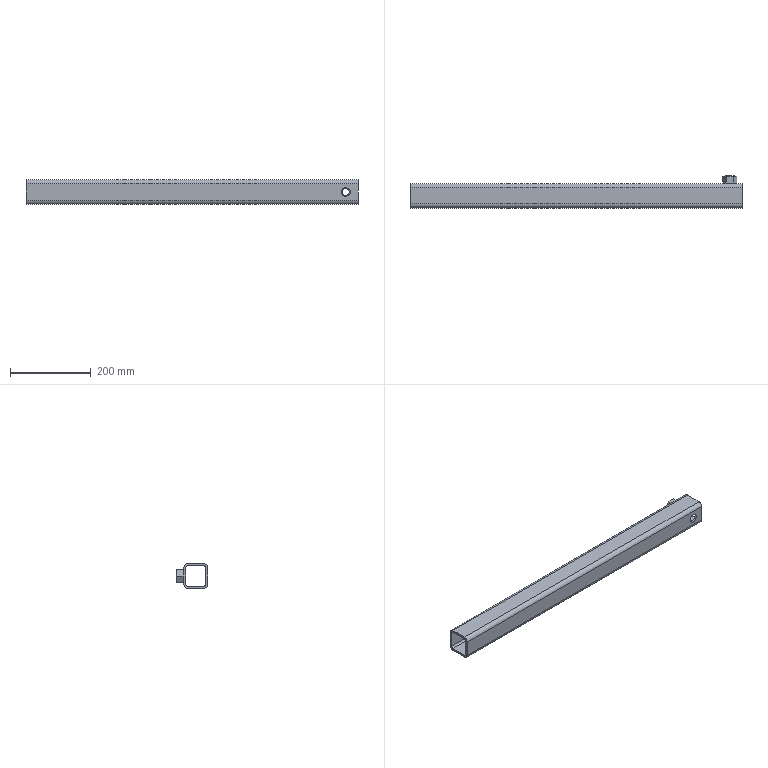Part | 2 solids | 36 faces | box 820 x 79 x 60 mm | volume 855655 mm3 | plane 18 | cylinder 14 | cone 4 | commonest cylinder face diameters 10 x4 20 x4 22 x4 17.294 x2
STEP:
#1=CARTESIAN_POINT('',(790.,25.,11.));
#2=VERTEX_POINT('',#1);
#3=CARTESIAN_POINT('',(790.,25.,-11.));
#4=VERTEX_POINT('',#3);
#5=CARTESIAN_POINT('',(790.,25.,0.));
#6=DIRECTION('',(0.,-1.,0.));
#7=DIRECTION('',(0.,0.,-1.));
#8=AXIS2_PLACEMENT_3D('',#5,#6,#7);
#9=CIRCLE('',#8,11.);
#10=EDGE_CURVE('',#2,#4,#9,.T.);
#11=ORIENTED_EDGE('',*,*,#10,.T.);
#12=CARTESIAN_POINT('',(790.,30.,-11.));
#13=VERTEX_POINT('',#12);
#14=CARTESIAN_POINT('',(790.,30.,-11.));
#15=DIRECTION('',(0.,1.,0.));
#16=VECTOR('',#15,1000.);
#17=LINE('',#14,#16);
#18=EDGE_CURVE('',#4,#13,#17,.T.);
#19=ORIENTED_EDGE('',*,*,#18,.T.);
#20=CARTESIAN_POINT('',(790.,30.,11.));
#21=VERTEX_POINT('',#20);
#22=CARTESIAN_POINT('',(790.,30.,0.));
#23=DIRECTION('',(0.,1.,0.));
#24=DIRECTION('',(0.,0.,1.));
#25=AXIS2_PLACEMENT_3D('',#22,#23,#24);
#26=CIRCLE('',#25,11.);
#27=EDGE_CURVE('',#13,#21,#26,.T.);
#28=ORIENTED_EDGE('',*,*,#27,.T.);
#29=CARTESIAN_POINT('',(790.,30.,11.));
#30=DIRECTION('',(0.,1.,0.));
#31=VECTOR('',#30,1000.);
#32=LINE('',#29,#31);
#33=EDGE_CURVE('',#2,#21,#32,.T.);
#34=ORIENTED_EDGE('',*,*,#33,.F.);
#35=EDGE_LOOP('',(#11,#19,#28,#34));
#36=FACE_OUTER_BOUND('',#35,.T.);
#37=CARTESIAN_POINT('',(790.,30.,0.));
#38=DIRECTION('',(0.,1.,0.));
#39=DIRECTION('',(0.,0.,1.));
#40=AXIS2_PLACEMENT_3D('',#37,#38,#39);
#41=CYLINDRICAL_SURFACE('',#40,11.);
#42=ADVANCED_FACE('',(#36),#41,.F.);
#43=CARTESIAN_POINT('',(790.,-30.,-11.));
#44=VERTEX_POINT('',#43);
#45=CARTESIAN_POINT('',(790.,-30.,11.));
#46=VERTEX_POINT('',#45);
#47=CARTESIAN_POINT('',(790.,-30.,0.));
#48=DIRECTION('',(0.,1.,0.));
#49=DIRECTION('',(0.,0.,1.));
#50=AXIS2_PLACEMENT_3D('',#47,#48,#49);
#51=CIRCLE('',#50,11.);
#52=EDGE_CURVE('',#44,#46,#51,.T.);
#53=ORIENTED_EDGE('',*,*,#52,.F.);
#54=CARTESIAN_POINT('',(790.,-25.,-11.));
#55=VERTEX_POINT('',#54);
#56=CARTESIAN_POINT('',(790.,30.,-11.));
#57=DIRECTION('',(0.,1.,0.));
#58=VECTOR('',#57,1000.);
#59=LINE('',#56,#58);
#60=EDGE_CURVE('',#44,#55,#59,.T.);
#61=ORIENTED_EDGE('',*,*,#60,.T.);
#62=CARTESIAN_POINT('',(790.,-25.,11.));
#63=VERTEX_POINT('',#62);
#64=CARTESIAN_POINT('',(790.,-25.,0.));
#65=DIRECTION('',(0.,1.,0.));
#66=DIRECTION('',(0.,0.,1.));
#67=AXIS2_PLACEMENT_3D('',#64,#65,#66);
#68=CIRCLE('',#67,11.);
#69=EDGE_CURVE('',#55,#63,#68,.T.);
#70=ORIENTED_EDGE('',*,*,#69,.T.);
#71=CARTESIAN_POINT('',(790.,30.,11.));
#72=DIRECTION('',(0.,1.,0.));
#73=VECTOR('',#72,1000.);
#74=LINE('',#71,#73);
#75=EDGE_CURVE('',#46,#63,#74,.T.);
#76=ORIENTED_EDGE('',*,*,#75,.F.);
#77=EDGE_LOOP('',(#53,#61,#70,#76));
#78=FACE_OUTER_BOUND('',#77,.T.);
#79=CARTESIAN_POINT('',(790.,30.,0.));
#80=DIRECTION('',(0.,1.,0.));
#81=DIRECTION('',(0.,0.,1.));
#82=AXIS2_PLACEMENT_3D('',#79,#80,#81);
#83=CYLINDRICAL_SURFACE('',#82,11.);
#84=ADVANCED_FACE('',(#78),#83,.F.);
#85=CARTESIAN_POINT('',(0.,20.,-30.));
#86=VERTEX_POINT('',#85);
#87=CARTESIAN_POINT('',(0.,30.,-20.));
#88=VERTEX_POINT('',#87);
#89=CARTESIAN_POINT('',(0.,20.,-20.));
#90=DIRECTION('',(1.,0.,0.));
#91=DIRECTION('',(0.,0.,-1.));
#92=AXIS2_PLACEMENT_3D('',#89,#90,#91);
#93=CIRCLE('',#92,10.);
#94=EDGE_CURVE('',#86,#88,#93,.T.);
#95=ORIENTED_EDGE('',*,*,#94,.T.);
#96=CARTESIAN_POINT('',(820.,30.,-20.));
#97=VERTEX_POINT('',#96);
#98=CARTESIAN_POINT('',(820.,30.,-20.));
#99=DIRECTION('',(-1.,0.,0.));
#100=VECTOR('',#99,1000.);
#101=LINE('',#98,#100);
#102=EDGE_CURVE('',#97,#88,#101,.T.);
#103=ORIENTED_EDGE('',*,*,#102,.F.);
#104=CARTESIAN_POINT('',(820.,20.,-30.));
#105=VERTEX_POINT('',#104);
#106=CARTESIAN_POINT('',(820.,20.,-20.));
#107=DIRECTION('',(1.,0.,0.));
#108=DIRECTION('',(0.,0.,-1.));
#109=AXIS2_PLACEMENT_3D('',#106,#107,#108);
#110=CIRCLE('',#109,10.);
#111=EDGE_CURVE('',#105,#97,#110,.T.);
#112=ORIENTED_EDGE('',*,*,#111,.F.);
#113=CARTESIAN_POINT('',(820.,20.,-30.));
#114=DIRECTION('',(-1.,0.,0.));
#115=VECTOR('',#114,1000.);
#116=LINE('',#113,#115);
#117=EDGE_CURVE('',#105,#86,#116,.T.);
#118=ORIENTED_EDGE('',*,*,#117,.T.);
#119=EDGE_LOOP('',(#95,#103,#112,#118));
#120=FACE_OUTER_BOUND('',#119,.T.);
#121=CARTESIAN_POINT('',(820.,20.,-20.));
#122=DIRECTION('',(-1.,0.,0.));
#123=DIRECTION('',(0.,0.,1.));
#124=AXIS2_PLACEMENT_3D('',#121,#122,#123);
#125=CYLINDRICAL_SURFACE('',#124,10.);
#126=ADVANCED_FACE('',(#120),#125,.T.);
#127=CARTESIAN_POINT('',(790.,30.,0.));
#128=DIRECTION('',(0.,1.,0.));
#129=DIRECTION('',(0.,0.,1.));
#130=AXIS2_PLACEMENT_3D('',#127,#128,#129);
#131=CIRCLE('',#130,11.);
#132=EDGE_CURVE('',#21,#13,#131,.T.);
#133=ORIENTED_EDGE('',*,*,#132,.F.);
#134=ORIENTED_EDGE('',*,*,#27,.F.);
#135=EDGE_LOOP('',(#133,#134));
#136=FACE_BOUND('',#135,.T.);
#137=CARTESIAN_POINT('',(0.,30.,20.));
#138=VERTEX_POINT('',#137);
#139=CARTESIAN_POINT('',(0.,30.,-20.));
#140=DIRECTION('',(0.,0.,1.));
#141=VECTOR('',#140,1000.);
#142=LINE('',#139,#141);
#143=EDGE_CURVE('',#88,#138,#142,.T.);
#144=ORIENTED_EDGE('',*,*,#143,.T.);
#145=CARTESIAN_POINT('',(820.,30.,20.));
#146=VERTEX_POINT('',#145);
#147=CARTESIAN_POINT('',(820.,30.,20.));
#148=DIRECTION('',(-1.,0.,0.));
#149=VECTOR('',#148,1000.);
#150=LINE('',#147,#149);
#151=EDGE_CURVE('',#146,#138,#150,.T.);
#152=ORIENTED_EDGE('',*,*,#151,.F.);
#153=CARTESIAN_POINT('',(820.,30.,-20.));
#154=DIRECTION('',(0.,0.,1.));
#155=VECTOR('',#154,1000.);
#156=LINE('',#153,#155);
#157=EDGE_CURVE('',#97,#146,#156,.T.);
#158=ORIENTED_EDGE('',*,*,#157,.F.);
#159=ORIENTED_EDGE('',*,*,#102,.T.);
#160=EDGE_LOOP('',(#144,#152,#158,#159));
#161=FACE_OUTER_BOUND('',#160,.T.);
#162=CARTESIAN_POINT('',(820.,30.,-20.));
#163=DIRECTION('',(0.,-1.,0.));
#164=DIRECTION('',(0.,0.,-1.));
#165=AXIS2_PLACEMENT_3D('',#162,#163,#164);
#166=PLANE('',#165);
#167=ADVANCED_FACE('',(#136,#161),#166,.F.);
#168=CARTESIAN_POINT('',(0.,20.,30.));
#169=VERTEX_POINT('',#168);
#170=CARTESIAN_POINT('',(0.,20.,20.));
#171=DIRECTION('',(1.,0.,0.));
#172=DIRECTION('',(0.,0.,-1.));
#173=AXIS2_PLACEMENT_3D('',#170,#171,#172);
#174=CIRCLE('',#173,10.);
#175=EDGE_CURVE('',#138,#169,#174,.T.);
#176=ORIENTED_EDGE('',*,*,#175,.T.);
#177=CARTESIAN_POINT('',(820.,20.,30.));
#178=VERTEX_POINT('',#177);
#179=CARTESIAN_POINT('',(820.,20.,30.));
#180=DIRECTION('',(-1.,0.,0.));
#181=VECTOR('',#180,1000.);
#182=LINE('',#179,#181);
#183=EDGE_CURVE('',#178,#169,#182,.T.);
#184=ORIENTED_EDGE('',*,*,#183,.F.);
#185=CARTESIAN_POINT('',(820.,20.,20.));
#186=DIRECTION('',(1.,0.,0.));
#187=DIRECTION('',(0.,0.,-1.));
#188=AXIS2_PLACEMENT_3D('',#185,#186,#187);
#189=CIRCLE('',#188,10.);
#190=EDGE_CURVE('',#146,#178,#189,.T.);
#191=ORIENTED_EDGE('',*,*,#190,.F.);
#192=ORIENTED_EDGE('',*,*,#151,.T.);
#193=EDGE_LOOP('',(#176,#184,#191,#192));
#194=FACE_OUTER_BOUND('',#193,.T.);
#195=CARTESIAN_POINT('',(820.,20.,20.));
#196=DIRECTION('',(-1.,0.,0.));
#197=DIRECTION('',(0.,0.,1.));
#198=AXIS2_PLACEMENT_3D('',#195,#196,#197);
#199=CYLINDRICAL_SURFACE('',#198,10.);
#200=ADVANCED_FACE('',(#194),#199,.T.);
#201=CARTESIAN_POINT('',(0.,-20.,30.));
#202=VERTEX_POINT('',#201);
#203=CARTESIAN_POINT('',(0.,-20.,30.));
#204=DIRECTION('',(0.,-1.,0.));
#205=VECTOR('',#204,1000.);
#206=LINE('',#203,#205);
#207=EDGE_CURVE('',#169,#202,#206,.T.);
#208=ORIENTED_EDGE('',*,*,#207,.T.);
#209=CARTESIAN_POINT('',(820.,-20.,30.));
#210=VERTEX_POINT('',#209);
#211=CARTESIAN_POINT('',(820.,-20.,30.));
#212=DIRECTION('',(-1.,0.,0.));
#213=VECTOR('',#212,1000.);
#214=LINE('',#211,#213);
#215=EDGE_CURVE('',#210,#202,#214,.T.);
#216=ORIENTED_EDGE('',*,*,#215,.F.);
#217=CARTESIAN_POINT('',(820.,-20.,30.));
#218=DIRECTION('',(0.,-1.,0.));
#219=VECTOR('',#218,1000.);
#220=LINE('',#217,#219);
#221=EDGE_CURVE('',#178,#210,#220,.T.);
#222=ORIENTED_EDGE('',*,*,#221,.F.);
#223=ORIENTED_EDGE('',*,*,#183,.T.);
#224=EDGE_LOOP('',(#208,#216,#222,#223));
#225=FACE_OUTER_BOUND('',#224,.T.);
#226=CARTESIAN_POINT('',(820.,-20.,30.));
#227=DIRECTION('',(0.,0.,-1.));
#228=DIRECTION('',(-1.,0.,0.));
#229=AXIS2_PLACEMENT_3D('',#226,#227,#228);
#230=PLANE('',#229);
#231=ADVANCED_FACE('',(#225),#230,.F.);
#232=CARTESIAN_POINT('',(0.,-30.,20.));
#233=VERTEX_POINT('',#232);
#234=CARTESIAN_POINT('',(0.,-20.,20.));
#235=DIRECTION('',(1.,0.,0.));
#236=DIRECTION('',(0.,0.,-1.));
#237=AXIS2_PLACEMENT_3D('',#234,#235,#236);
#238=CIRCLE('',#237,10.);
#239=EDGE_CURVE('',#202,#233,#238,.T.);
#240=ORIENTED_EDGE('',*,*,#239,.T.);
#241=CARTESIAN_POINT('',(820.,-30.,20.));
#242=VERTEX_POINT('',#241);
#243=CARTESIAN_POINT('',(820.,-30.,20.));
#244=DIRECTION('',(-1.,0.,0.));
#245=VECTOR('',#244,1000.);
#246=LINE('',#243,#245);
#247=EDGE_CURVE('',#242,#233,#246,.T.);
#248=ORIENTED_EDGE('',*,*,#247,.F.);
#249=CARTESIAN_POINT('',(820.,-20.,20.));
#250=DIRECTION('',(1.,0.,0.));
#251=DIRECTION('',(0.,0.,-1.));
#252=AXIS2_PLACEMENT_3D('',#249,#250,#251);
#253=CIRCLE('',#252,10.);
#254=EDGE_CURVE('',#210,#242,#253,.T.);
#255=ORIENTED_EDGE('',*,*,#254,.F.);
#256=ORIENTED_EDGE('',*,*,#215,.T.);
#257=EDGE_LOOP('',(#240,#248,#255,#256));
#258=FACE_OUTER_BOUND('',#257,.T.);
#259=CARTESIAN_POINT('',(820.,-20.,20.));
#260=DIRECTION('',(-1.,0.,0.));
#261=DIRECTION('',(0.,0.,1.));
#262=AXIS2_PLACEMENT_3D('',#259,#260,#261);
#263=CYLINDRICAL_SURFACE('',#262,10.);
#264=ADVANCED_FACE('',(#258),#263,.T.);
#265=CARTESIAN_POINT('',(790.,-30.,0.));
#266=DIRECTION('',(0.,1.,0.));
#267=DIRECTION('',(0.,0.,1.));
#268=AXIS2_PLACEMENT_3D('',#265,#266,#267);
#269=CIRCLE('',#268,11.);
#270=EDGE_CURVE('',#46,#44,#269,.T.);
#271=ORIENTED_EDGE('',*,*,#270,.T.);
#272=ORIENTED_EDGE('',*,*,#52,.T.);
#273=EDGE_LOOP('',(#271,#272));
#274=FACE_BOUND('',#273,.T.);
#275=CARTESIAN_POINT('',(0.,-30.,-20.));
#276=VERTEX_POINT('',#275);
#277=CARTESIAN_POINT('',(0.,-30.,20.));
#278=DIRECTION('',(0.,0.,-1.));
#279=VECTOR('',#278,1000.);
#280=LINE('',#277,#279);
#281=EDGE_CURVE('',#233,#276,#280,.T.);
#282=ORIENTED_EDGE('',*,*,#281,.T.);
#283=CARTESIAN_POINT('',(820.,-30.,-20.));
#284=VERTEX_POINT('',#283);
#285=CARTESIAN_POINT('',(820.,-30.,-20.));
#286=DIRECTION('',(-1.,0.,0.));
#287=VECTOR('',#286,1000.);
#288=LINE('',#285,#287);
#289=EDGE_CURVE('',#284,#276,#288,.T.);
#290=ORIENTED_EDGE('',*,*,#289,.F.);
#291=CARTESIAN_POINT('',(820.,-30.,20.));
#292=DIRECTION('',(0.,0.,-1.));
#293=VECTOR('',#292,1000.);
#294=LINE('',#291,#293);
#295=EDGE_CURVE('',#242,#284,#294,.T.);
#296=ORIENTED_EDGE('',*,*,#295,.F.);
#297=ORIENTED_EDGE('',*,*,#247,.T.);
#298=EDGE_LOOP('',(#282,#290,#296,#297));
#299=FACE_OUTER_BOUND('',#298,.T.);
#300=CARTESIAN_POINT('',(820.,-30.,20.));
#301=DIRECTION('',(0.,1.,0.));
#302=DIRECTION('',(0.,0.,1.));
#303=AXIS2_PLACEMENT_3D('',#300,#301,#302);
#304=PLANE('',#303);
#305=ADVANCED_FACE('',(#274,#299),#304,.F.);
#306=CARTESIAN_POINT('',(0.,-20.,-30.));
#307=VERTEX_POINT('',#306);
#308=CARTESIAN_POINT('',(0.,-20.,-20.));
#309=DIRECTION('',(1.,0.,0.));
#310=DIRECTION('',(0.,0.,-1.));
#311=AXIS2_PLACEMENT_3D('',#308,#309,#310);
#312=CIRCLE('',#311,10.);
#313=EDGE_CURVE('',#276,#307,#312,.T.);
#314=ORIENTED_EDGE('',*,*,#313,.T.);
#315=CARTESIAN_POINT('',(820.,-20.,-30.));
#316=VERTEX_POINT('',#315);
#317=CARTESIAN_POINT('',(820.,-20.,-30.));
#318=DIRECTION('',(-1.,0.,0.));
#319=VECTOR('',#318,1000.);
#320=LINE('',#317,#319);
#321=EDGE_CURVE('',#316,#307,#320,.T.);
#322=ORIENTED_EDGE('',*,*,#321,.F.);
#323=CARTESIAN_POINT('',(820.,-20.,-20.));
#324=DIRECTION('',(1.,0.,0.));
#325=DIRECTION('',(0.,0.,-1.));
#326=AXIS2_PLACEMENT_3D('',#323,#324,#325);
#327=CIRCLE('',#326,10.);
#328=EDGE_CURVE('',#284,#316,#327,.T.);
#329=ORIENTED_EDGE('',*,*,#328,.F.);
#330=ORIENTED_EDGE('',*,*,#289,.T.);
#331=EDGE_LOOP('',(#314,#322,#329,#330));
#332=FACE_OUTER_BOUND('',#331,.T.);
#333=CARTESIAN_POINT('',(820.,-20.,-20.));
#334=DIRECTION('',(-1.,0.,0.));
#335=DIRECTION('',(0.,0.,1.));
#336=AXIS2_PLACEMENT_3D('',#333,#334,#335);
#337=CYLINDRICAL_SURFACE('',#336,10.);
#338=ADVANCED_FACE('',(#332),#337,.T.);
#339=CARTESIAN_POINT('',(0.,25.,20.));
#340=VERTEX_POINT('',#339);
#341=CARTESIAN_POINT('',(0.,20.,25.));
#342=VERTEX_POINT('',#341);
#343=CARTESIAN_POINT('',(0.,20.,20.));
#344=DIRECTION('',(1.,0.,0.));
#345=DIRECTION('',(0.,0.,-1.));
#346=AXIS2_PLACEMENT_3D('',#343,#344,#345);
#347=CIRCLE('',#346,5.);
#348=EDGE_CURVE('',#340,#342,#347,.T.);
#349=ORIENTED_EDGE('',*,*,#348,.F.);
#350=CARTESIAN_POINT('',(820.,25.,20.));
#351=VERTEX_POINT('',#350);
#352=CARTESIAN_POINT('',(820.,25.,20.));
#353=DIRECTION('',(-1.,0.,0.));
#354=VECTOR('',#353,1000.);
#355=LINE('',#352,#354);
#356=EDGE_CURVE('',#351,#340,#355,.T.);
#357=ORIENTED_EDGE('',*,*,#356,.F.);
#358=CARTESIAN_POINT('',(820.,20.,25.));
#359=VERTEX_POINT('',#358);
#360=CARTESIAN_POINT('',(820.,20.,20.));
#361=DIRECTION('',(1.,0.,0.));
#362=DIRECTION('',(0.,0.,-1.));
#363=AXIS2_PLACEMENT_3D('',#360,#361,#362);
#364=CIRCLE('',#363,5.);
#365=EDGE_CURVE('',#351,#359,#364,.T.);
#366=ORIENTED_EDGE('',*,*,#365,.T.);
#367=CARTESIAN_POINT('',(820.,20.,25.));
#368=DIRECTION('',(-1.,0.,0.));
#369=VECTOR('',#368,1000.);
#370=LINE('',#367,#369);
#371=EDGE_CURVE('',#359,#342,#370,.T.);
#372=ORIENTED_EDGE('',*,*,#371,.T.);
#373=EDGE_LOOP('',(#349,#357,#366,#372));
#374=FACE_OUTER_BOUND('',#373,.T.);
#375=CARTESIAN_POINT('',(820.,20.,20.));
#376=DIRECTION('',(-1.,0.,0.));
#377=DIRECTION('',(0.,0.,1.));
#378=AXIS2_PLACEMENT_3D('',#375,#376,#377);
#379=CYLINDRICAL_SURFACE('',#378,5.);
#380=ADVANCED_FACE('',(#374),#379,.F.);
#381=ORIENTED_EDGE('',*,*,#10,.F.);
#382=CARTESIAN_POINT('',(790.,25.,0.));
#383=DIRECTION('',(0.,-1.,0.));
#384=DIRECTION('',(0.,0.,-1.));
#385=AXIS2_PLACEMENT_3D('',#382,#383,#384);
#386=CIRCLE('',#385,11.);
#387=EDGE_CURVE('',#4,#2,#386,.T.);
#388=ORIENTED_EDGE('',*,*,#387,.F.);
#389=EDGE_LOOP('',(#381,#388));
#390=FACE_BOUND('',#389,.T.);
#391=CARTESIAN_POINT('',(0.,25.,-20.));
#392=VERTEX_POINT('',#391);
#393=CARTESIAN_POINT('',(0.,25.,-20.));
#394=DIRECTION('',(0.,0.,1.));
#395=VECTOR('',#394,1000.);
#396=LINE('',#393,#395);
#397=EDGE_CURVE('',#392,#340,#396,.T.);
#398=ORIENTED_EDGE('',*,*,#397,.F.);
#399=CARTESIAN_POINT('',(820.,25.,-20.));
#400=VERTEX_POINT('',#399);
#401=CARTESIAN_POINT('',(820.,25.,-20.));
#402=DIRECTION('',(-1.,0.,0.));
#403=VECTOR('',#402,1000.);
#404=LINE('',#401,#403);
#405=EDGE_CURVE('',#400,#392,#404,.T.);
#406=ORIENTED_EDGE('',*,*,#405,.F.);
#407=CARTESIAN_POINT('',(820.,25.,-20.));
#408=DIRECTION('',(0.,0.,1.));
#409=VECTOR('',#408,1000.);
#410=LINE('',#407,#409);
#411=EDGE_CURVE('',#400,#351,#410,.T.);
#412=ORIENTED_EDGE('',*,*,#411,.T.);
#413=ORIENTED_EDGE('',*,*,#356,.T.);
#414=EDGE_LOOP('',(#398,#406,#412,#413));
#415=FACE_OUTER_BOUND('',#414,.T.);
#416=CARTESIAN_POINT('',(820.,25.,-20.));
#417=DIRECTION('',(0.,-1.,0.));
#418=DIRECTION('',(0.,0.,-1.));
#419=AXIS2_PLACEMENT_3D('',#416,#417,#418);
#420=PLANE('',#419);
#421=ADVANCED_FACE('',(#390,#415),#420,.T.);
#422=CARTESIAN_POINT('',(0.,20.,-25.));
#423=VERTEX_POINT('',#422);
#424=CARTESIAN_POINT('',(0.,20.,-20.));
#425=DIRECTION('',(1.,0.,0.));
#426=DIRECTION('',(0.,0.,-1.));
#427=AXIS2_PLACEMENT_3D('',#424,#425,#426);
#428=CIRCLE('',#427,5.);
#429=EDGE_CURVE('',#423,#392,#428,.T.);
#430=ORIENTED_EDGE('',*,*,#429,.F.);
#431=CARTESIAN_POINT('',(820.,20.,-25.));
#432=VERTEX_POINT('',#431);
#433=CARTESIAN_POINT('',(820.,20.,-25.));
#434=DIRECTION('',(-1.,0.,0.));
#435=VECTOR('',#434,1000.);
#436=LINE('',#433,#435);
#437=EDGE_CURVE('',#432,#423,#436,.T.);
#438=ORIENTED_EDGE('',*,*,#437,.F.);
#439=CARTESIAN_POINT('',(820.,20.,-20.));
#440=DIRECTION('',(1.,0.,0.));
#441=DIRECTION('',(0.,0.,-1.));
#442=AXIS2_PLACEMENT_3D('',#439,#440,#441);
#443=CIRCLE('',#442,5.);
#444=EDGE_CURVE('',#432,#400,#443,.T.);
#445=ORIENTED_EDGE('',*,*,#444,.T.);
#446=ORIENTED_EDGE('',*,*,#405,.T.);
#447=EDGE_LOOP('',(#430,#438,#445,#446));
#448=FACE_OUTER_BOUND('',#447,.T.);
#449=CARTESIAN_POINT('',(820.,20.,-20.));
#450=DIRECTION('',(-1.,0.,0.));
#451=DIRECTION('',(0.,0.,1.));
#452=AXIS2_PLACEMENT_3D('',#449,#450,#451);
#453=CYLINDRICAL_SURFACE('',#452,5.);
#454=ADVANCED_FACE('',(#448),#453,.F.);
#455=CARTESIAN_POINT('',(0.,-20.,-25.));
#456=VERTEX_POINT('',#455);
#457=CARTESIAN_POINT('',(0.,20.,-25.));
#458=DIRECTION('',(0.,1.,0.));
#459=VECTOR('',#458,1000.);
#460=LINE('',#457,#459);
#461=EDGE_CURVE('',#456,#423,#460,.T.);
#462=ORIENTED_EDGE('',*,*,#461,.F.);
#463=CARTESIAN_POINT('',(820.,-20.,-25.));
#464=VERTEX_POINT('',#463);
#465=CARTESIAN_POINT('',(820.,-20.,-25.));
#466=DIRECTION('',(-1.,0.,0.));
#467=VECTOR('',#466,1000.);
#468=LINE('',#465,#467);
#469=EDGE_CURVE('',#464,#456,#468,.T.);
#470=ORIENTED_EDGE('',*,*,#469,.F.);
#471=CARTESIAN_POINT('',(820.,20.,-25.));
#472=DIRECTION('',(0.,1.,0.));
#473=VECTOR('',#472,1000.);
#474=LINE('',#471,#473);
#475=EDGE_CURVE('',#464,#432,#474,.T.);
#476=ORIENTED_EDGE('',*,*,#475,.T.);
#477=ORIENTED_EDGE('',*,*,#437,.T.);
#478=EDGE_LOOP('',(#462,#470,#476,#477));
#479=FACE_OUTER_BOUND('',#478,.T.);
#480=CARTESIAN_POINT('',(820.,20.,-25.));
#481=DIRECTION('',(0.,0.,1.));
#482=DIRECTION('',(1.,0.,0.));
#483=AXIS2_PLACEMENT_3D('',#480,#481,#482);
#484=PLANE('',#483);
#485=ADVANCED_FACE('',(#479),#484,.T.);
#486=CARTESIAN_POINT('',(0.,-25.,-20.));
#487=VERTEX_POINT('',#486);
#488=CARTESIAN_POINT('',(0.,-20.,-20.));
#489=DIRECTION('',(1.,0.,0.));
#490=DIRECTION('',(0.,0.,-1.));
#491=AXIS2_PLACEMENT_3D('',#488,#489,#490);
#492=CIRCLE('',#491,5.);
#493=EDGE_CURVE('',#487,#456,#492,.T.);
#494=ORIENTED_EDGE('',*,*,#493,.F.);
#495=CARTESIAN_POINT('',(820.,-25.,-20.));
#496=VERTEX_POINT('',#495);
#497=CARTESIAN_POINT('',(820.,-25.,-20.));
#498=DIRECTION('',(-1.,0.,0.));
#499=VECTOR('',#498,1000.);
#500=LINE('',#497,#499);
#501=EDGE_CURVE('',#496,#487,#500,.T.);
#502=ORIENTED_EDGE('',*,*,#501,.F.);
#503=CARTESIAN_POINT('',(820.,-20.,-20.));
#504=DIRECTION('',(1.,0.,0.));
#505=DIRECTION('',(0.,0.,-1.));
#506=AXIS2_PLACEMENT_3D('',#503,#504,#505);
#507=CIRCLE('',#506,5.);
#508=EDGE_CURVE('',#496,#464,#507,.T.);
#509=ORIENTED_EDGE('',*,*,#508,.T.);
#510=ORIENTED_EDGE('',*,*,#469,.T.);
#511=EDGE_LOOP('',(#494,#502,#509,#510));
#512=FACE_OUTER_BOUND('',#511,.T.);
#513=CARTESIAN_POINT('',(820.,-20.,-20.));
#514=DIRECTION('',(-1.,0.,0.));
#515=DIRECTION('',(0.,0.,1.));
#516=AXIS2_PLACEMENT_3D('',#513,#514,#515);
#517=CYLINDRICAL_SURFACE('',#516,5.);
#518=ADVANCED_FACE('',(#512),#517,.F.);
#519=CARTESIAN_POINT('',(790.,-25.,0.));
#520=DIRECTION('',(0.,1.,0.));
#521=DIRECTION('',(0.,0.,1.));
#522=AXIS2_PLACEMENT_3D('',#519,#520,#521);
#523=CIRCLE('',#522,11.);
#524=EDGE_CURVE('',#63,#55,#523,.T.);
#525=ORIENTED_EDGE('',*,*,#524,.F.);
#526=ORIENTED_EDGE('',*,*,#69,.F.);
#527=EDGE_LOOP('',(#525,#526));
#528=FACE_BOUND('',#527,.T.);
#529=CARTESIAN_POINT('',(0.,-25.,20.));
#530=VERTEX_POINT('',#529);
#531=CARTESIAN_POINT('',(0.,-25.,20.));
#532=DIRECTION('',(0.,0.,-1.));
#533=VECTOR('',#532,1000.);
#534=LINE('',#531,#533);
#535=EDGE_CURVE('',#530,#487,#534,.T.);
#536=ORIENTED_EDGE('',*,*,#535,.F.);
#537=CARTESIAN_POINT('',(820.,-25.,20.));
#538=VERTEX_POINT('',#537);
#539=CARTESIAN_POINT('',(820.,-25.,20.));
#540=DIRECTION('',(-1.,0.,0.));
#541=VECTOR('',#540,1000.);
#542=LINE('',#539,#541);
#543=EDGE_CURVE('',#538,#530,#542,.T.);
#544=ORIENTED_EDGE('',*,*,#543,.F.);
#545=CARTESIAN_POINT('',(820.,-25.,20.));
#546=DIRECTION('',(0.,0.,-1.));
#547=VECTOR('',#546,1000.);
#548=LINE('',#545,#547);
#549=EDGE_CURVE('',#538,#496,#548,.T.);
#550=ORIENTED_EDGE('',*,*,#549,.T.);
#551=ORIENTED_EDGE('',*,*,#501,.T.);
#552=EDGE_LOOP('',(#536,#544,#550,#551));
#553=FACE_OUTER_BOUND('',#552,.T.);
#554=CARTESIAN_POINT('',(820.,-25.,20.));
#555=DIRECTION('',(0.,1.,0.));
#556=DIRECTION('',(0.,0.,1.));
#557=AXIS2_PLACEMENT_3D('',#554,#555,#556);
#558=PLANE('',#557);
#559=ADVANCED_FACE('',(#528,#553),#558,.T.);
#560=CARTESIAN_POINT('',(0.,-20.,25.));
#561=VERTEX_POINT('',#560);
#562=CARTESIAN_POINT('',(0.,-20.,20.));
#563=DIRECTION('',(1.,0.,0.));
#564=DIRECTION('',(0.,0.,-1.));
#565=AXIS2_PLACEMENT_3D('',#562,#563,#564);
#566=CIRCLE('',#565,5.);
#567=EDGE_CURVE('',#561,#530,#566,.T.);
#568=ORIENTED_EDGE('',*,*,#567,.F.);
#569=CARTESIAN_POINT('',(820.,-20.,25.));
#570=VERTEX_POINT('',#569);
#571=CARTESIAN_POINT('',(820.,-20.,25.));
#572=DIRECTION('',(-1.,0.,0.));
#573=VECTOR('',#572,1000.);
#574=LINE('',#571,#573);
#575=EDGE_CURVE('',#570,#561,#574,.T.);
#576=ORIENTED_EDGE('',*,*,#575,.F.);
#577=CARTESIAN_POINT('',(820.,-20.,20.));
#578=DIRECTION('',(1.,0.,0.));
#579=DIRECTION('',(0.,0.,-1.));
#580=AXIS2_PLACEMENT_3D('',#577,#578,#579);
#581=CIRCLE('',#580,5.);
#582=EDGE_CURVE('',#570,#538,#581,.T.);
#583=ORIENTED_EDGE('',*,*,#582,.T.);
#584=ORIENTED_EDGE('',*,*,#543,.T.);
#585=EDGE_LOOP('',(#568,#576,#583,#584));
#586=FACE_OUTER_BOUND('',#585,.T.);
#587=CARTESIAN_POINT('',(820.,-20.,20.));
#588=DIRECTION('',(-1.,0.,0.));
#589=DIRECTION('',(0.,0.,1.));
#590=AXIS2_PLACEMENT_3D('',#587,#588,#589);
#591=CYLINDRICAL_SURFACE('',#590,5.);
#592=ADVANCED_FACE('',(#586),#591,.F.);
#593=CARTESIAN_POINT('',(0.,-20.,25.));
#594=DIRECTION('',(0.,-1.,0.));
#595=VECTOR('',#594,1000.);
#596=LINE('',#593,#595);
#597=EDGE_CURVE('',#342,#561,#596,.T.);
#598=ORIENTED_EDGE('',*,*,#597,.F.);
#599=ORIENTED_EDGE('',*,*,#371,.F.);
#600=CARTESIAN_POINT('',(820.,-20.,25.));
#601=DIRECTION('',(0.,-1.,0.));
#602=VECTOR('',#601,1000.);
#603=LINE('',#600,#602);
#604=EDGE_CURVE('',#359,#570,#603,.T.);
#605=ORIENTED_EDGE('',*,*,#604,.T.);
#606=ORIENTED_EDGE('',*,*,#575,.T.);
#607=EDGE_LOOP('',(#598,#599,#605,#606));
#608=FACE_OUTER_BOUND('',#607,.T.);
#609=CARTESIAN_POINT('',(820.,-20.,25.));
#610=DIRECTION('',(0.,0.,-1.));
#611=DIRECTION('',(-1.,0.,0.));
#612=AXIS2_PLACEMENT_3D('',#609,#610,#611);
#613=PLANE('',#612);
#614=ADVANCED_FACE('',(#608),#613,.T.);
#615=CARTESIAN_POINT('',(0.,20.,-30.));
#616=DIRECTION('',(0.,1.,0.));
#617=VECTOR('',#616,1000.);
#618=LINE('',#615,#617);
#619=EDGE_CURVE('',#307,#86,#618,.T.);
#620=ORIENTED_EDGE('',*,*,#619,.T.);
#621=ORIENTED_EDGE('',*,*,#117,.F.);
#622=CARTESIAN_POINT('',(820.,20.,-30.));
#623=DIRECTION('',(0.,1.,0.));
#624=VECTOR('',#623,1000.);
#625=LINE('',#622,#624);
#626=EDGE_CURVE('',#316,#105,#625,.T.);
#627=ORIENTED_EDGE('',*,*,#626,.F.);
#628=ORIENTED_EDGE('',*,*,#321,.T.);
#629=EDGE_LOOP('',(#620,#621,#627,#628));
#630=FACE_OUTER_BOUND('',#629,.T.);
#631=CARTESIAN_POINT('',(820.,20.,-30.));
#632=DIRECTION('',(0.,0.,1.));
#633=DIRECTION('',(1.,0.,0.));
#634=AXIS2_PLACEMENT_3D('',#631,#632,#633);
#635=PLANE('',#634);
#636=ADVANCED_FACE('',(#630),#635,.F.);
#637=ORIENTED_EDGE('',*,*,#365,.F.);
#638=ORIENTED_EDGE('',*,*,#411,.F.);
#639=ORIENTED_EDGE('',*,*,#444,.F.);
#640=ORIENTED_EDGE('',*,*,#475,.F.);
#641=ORIENTED_EDGE('',*,*,#508,.F.);
#642=ORIENTED_EDGE('',*,*,#549,.F.);
#643=ORIENTED_EDGE('',*,*,#582,.F.);
#644=ORIENTED_EDGE('',*,*,#604,.F.);
#645=EDGE_LOOP('',(#637,#638,#639,#640,#641,#642,#643,#644));
#646=FACE_BOUND('',#645,.T.);
#647=ORIENTED_EDGE('',*,*,#111,.T.);
#648=ORIENTED_EDGE('',*,*,#157,.T.);
#649=ORIENTED_EDGE('',*,*,#190,.T.);
#650=ORIENTED_EDGE('',*,*,#221,.T.);
#651=ORIENTED_EDGE('',*,*,#254,.T.);
#652=ORIENTED_EDGE('',*,*,#295,.T.);
#653=ORIENTED_EDGE('',*,*,#328,.T.);
#654=ORIENTED_EDGE('',*,*,#626,.T.);
#655=EDGE_LOOP('',(#647,#648,#649,#650,#651,#652,#653,#654));
#656=FACE_OUTER_BOUND('',#655,.T.);
#657=CARTESIAN_POINT('',(820.,20.,-20.));
#658=DIRECTION('',(1.,0.,0.));
#659=DIRECTION('',(0.,0.,-1.));
#660=AXIS2_PLACEMENT_3D('',#657,#658,#659);
#661=PLANE('',#660);
#662=ADVANCED_FACE('',(#646,#656),#661,.T.);
#663=ORIENTED_EDGE('',*,*,#348,.T.);
#664=ORIENTED_EDGE('',*,*,#597,.T.);
#665=ORIENTED_EDGE('',*,*,#567,.T.);
#666=ORIENTED_EDGE('',*,*,#535,.T.);
#667=ORIENTED_EDGE('',*,*,#493,.T.);
#668=ORIENTED_EDGE('',*,*,#461,.T.);
#669=ORIENTED_EDGE('',*,*,#429,.T.);
#670=ORIENTED_EDGE('',*,*,#397,.T.);
#671=EDGE_LOOP('',(#663,#664,#665,#666,#667,#668,#669,#670));
#672=FACE_BOUND('',#671,.T.);
#673=ORIENTED_EDGE('',*,*,#94,.F.);
#674=ORIENTED_EDGE('',*,*,#619,.F.);
#675=ORIENTED_EDGE('',*,*,#313,.F.);
#676=ORIENTED_EDGE('',*,*,#281,.F.);
#677=ORIENTED_EDGE('',*,*,#239,.F.);
#678=ORIENTED_EDGE('',*,*,#207,.F.);
#679=ORIENTED_EDGE('',*,*,#175,.F.);
#680=ORIENTED_EDGE('',*,*,#143,.F.);
#681=EDGE_LOOP('',(#673,#674,#675,#676,#677,#678,#679,#680));
#682=FACE_OUTER_BOUND('',#681,.T.);
#683=CARTESIAN_POINT('',(0.,20.,-20.));
#684=DIRECTION('',(1.,0.,0.));
#685=DIRECTION('',(0.,0.,-1.));
#686=AXIS2_PLACEMENT_3D('',#683,#684,#685);
#687=PLANE('',#686);
#688=ADVANCED_FACE('',(#672,#682),#687,.F.);
#689=ORIENTED_EDGE('',*,*,#60,.F.);
#690=ORIENTED_EDGE('',*,*,#270,.F.);
#691=ORIENTED_EDGE('',*,*,#75,.T.);
#692=ORIENTED_EDGE('',*,*,#524,.T.);
#693=EDGE_LOOP('',(#689,#690,#691,#692));
#694=FACE_OUTER_BOUND('',#693,.T.);
#695=CARTESIAN_POINT('',(790.,30.,0.));
#696=DIRECTION('',(0.,1.,0.));
#697=DIRECTION('',(0.,0.,1.));
#698=AXIS2_PLACEMENT_3D('',#695,#696,#697);
#699=CYLINDRICAL_SURFACE('',#698,11.);
#700=ADVANCED_FACE('',(#694),#699,.F.);
#701=ORIENTED_EDGE('',*,*,#18,.F.);
#702=ORIENTED_EDGE('',*,*,#387,.T.);
#703=ORIENTED_EDGE('',*,*,#33,.T.);
#704=ORIENTED_EDGE('',*,*,#132,.T.);
#705=EDGE_LOOP('',(#701,#702,#703,#704));
#706=FACE_OUTER_BOUND('',#705,.T.);
#707=CARTESIAN_POINT('',(790.,30.,0.));
#708=DIRECTION('',(0.,1.,0.));
#709=DIRECTION('',(0.,0.,1.));
#710=AXIS2_PLACEMENT_3D('',#707,#708,#709);
#711=CYLINDRICAL_SURFACE('',#710,11.);
#712=ADVANCED_FACE('',(#706),#711,.F.);
#713=CLOSED_SHELL('',(#42,#84,#126,#167,#200,#231,#264,#305,#338,#380,#421,#454,#485,#518,#559,#592,#614,#636,#662,#688,#700,#712));
#714=MANIFOLD_SOLID_BREP('',#713);
#715=CARTESIAN_POINT('',(775.375,30.,0.));
#716=VERTEX_POINT('',#715);
#717=CARTESIAN_POINT('',(804.625,30.,0.));
#718=VERTEX_POINT('',#717);
#719=CARTESIAN_POINT('',(790.,30.,0.));
#720=DIRECTION('',(0.,1.,0.));
#721=DIRECTION('',(-1.,0.,0.));
#722=AXIS2_PLACEMENT_3D('',#719,#720,#721);
#723=CIRCLE('',#722,14.625);
#724=EDGE_CURVE('',#716,#718,#723,.T.);
#725=ORIENTED_EDGE('',*,*,#724,.T.);
#726=CARTESIAN_POINT('',(807.321,31.556,0.));
#727=VERTEX_POINT('',#726);
#728=CARTESIAN_POINT('',(804.625,30.,0.));
#729=DIRECTION('',(0.866,0.5,0.));
#730=VECTOR('',#729,1000.);
#731=LINE('',#728,#730);
#732=EDGE_CURVE('',#718,#727,#731,.T.);
#733=ORIENTED_EDGE('',*,*,#732,.T.);
#734=CARTESIAN_POINT('',(798.66,31.556,15.));
#735=VERTEX_POINT('',#734);
#736=CARTESIAN_POINT('',(807.321,31.556,0.));
#737=CARTESIAN_POINT('',(806.613,31.148,1.225));
#738=CARTESIAN_POINT('',(805.901,30.812,2.458));
#739=CARTESIAN_POINT('',(804.462,30.346,4.951));
#740=CARTESIAN_POINT('',(803.735,30.217,6.21));
#741=CARTESIAN_POINT('',(802.631,30.216,8.123));
#742=CARTESIAN_POINT('',(802.261,30.247,8.764));
#743=CARTESIAN_POINT('',(801.529,30.369,10.031));
#744=CARTESIAN_POINT('',(801.166,30.46,10.661));
#745=CARTESIAN_POINT('',(800.082,30.81,12.537));
#746=CARTESIAN_POINT('',(799.368,31.148,13.774));
#747=CARTESIAN_POINT('',(798.66,31.556,15.));
#748=B_SPLINE_CURVE_WITH_KNOTS('',3,(#736,#737,#738,#739,#740,#741,#742,#743,#744,#745,#746,#747),.UNSPECIFIED.,.F.,.F.,(4,2,2,2,2,4),(0.000000238,0.004373,0.008747,0.01093,0.01312,0.01749),.UNSPECIFIED.);
#749=EDGE_CURVE('',#727,#735,#748,.T.);
#750=ORIENTED_EDGE('',*,*,#749,.T.);
#751=CARTESIAN_POINT('',(781.34,31.556,15.));
#752=VERTEX_POINT('',#751);
#753=CARTESIAN_POINT('',(798.66,31.556,15.));
#754=CARTESIAN_POINT('',(797.26,31.152,15.));
#755=CARTESIAN_POINT('',(795.842,30.816,15.));
#756=CARTESIAN_POINT('',(793.673,30.463,15.));
#757=CARTESIAN_POINT('',(792.942,30.371,15.));
#758=CARTESIAN_POINT('',(791.469,30.248,15.));
#759=CARTESIAN_POINT('',(790.734,30.217,15.));
#760=CARTESIAN_POINT('',(788.539,30.216,15.));
#761=CARTESIAN_POINT('',(787.084,30.342,15.));
#762=CARTESIAN_POINT('',(784.915,30.692,15.));
#763=CARTESIAN_POINT('',(784.193,30.835,15.));
#764=CARTESIAN_POINT('',(782.755,31.166,15.));
#765=CARTESIAN_POINT('',(782.044,31.353,15.));
#766=CARTESIAN_POINT('',(781.34,31.556,15.));
#767=B_SPLINE_CURVE_WITH_KNOTS('',3,(#753,#754,#755,#756,#757,#758,#759,#760,#761,#762,#763,#764,#765,#766),.UNSPECIFIED.,.F.,.F.,(4,2,2,2,2,2,4),(0.006384,0.01075,0.01294,0.01513,0.0195,0.02168,0.02387),.UNSPECIFIED.);
#768=EDGE_CURVE('',#735,#752,#767,.T.);
#769=ORIENTED_EDGE('',*,*,#768,.T.);
#770=CARTESIAN_POINT('',(772.679,31.556,0.));
#771=VERTEX_POINT('',#770);
#772=CARTESIAN_POINT('',(781.34,31.556,15.));
#773=CARTESIAN_POINT('',(780.633,31.148,13.775));
#774=CARTESIAN_POINT('',(779.921,30.812,12.542));
#775=CARTESIAN_POINT('',(778.481,30.346,10.049));
#776=CARTESIAN_POINT('',(777.754,30.217,8.79));
#777=CARTESIAN_POINT('',(776.65,30.216,6.877));
#778=CARTESIAN_POINT('',(776.28,30.247,6.236));
#779=CARTESIAN_POINT('',(775.548,30.369,4.969));
#780=CARTESIAN_POINT('',(775.185,30.46,4.339));
#781=CARTESIAN_POINT('',(774.101,30.81,2.463));
#782=CARTESIAN_POINT('',(773.387,31.148,1.226));
#783=CARTESIAN_POINT('',(772.679,31.556,0.));
#784=B_SPLINE_CURVE_WITH_KNOTS('',3,(#772,#773,#774,#775,#776,#777,#778,#779,#780,#781,#782,#783),.UNSPECIFIED.,.F.,.F.,(4,2,2,2,2,4),(0.000000238,0.004373,0.008747,0.01093,0.01312,0.01749),.UNSPECIFIED.);
#785=EDGE_CURVE('',#752,#771,#784,.T.);
#786=ORIENTED_EDGE('',*,*,#785,.T.);
#787=CARTESIAN_POINT('',(775.375,30.,0.));
#788=DIRECTION('',(-0.866,0.5,0.));
#789=VECTOR('',#788,1000.);
#790=LINE('',#787,#789);
#791=EDGE_CURVE('',#716,#771,#790,.T.);
#792=ORIENTED_EDGE('',*,*,#791,.F.);
#793=EDGE_LOOP('',(#725,#733,#750,#769,#786,#792));
#794=FACE_OUTER_BOUND('',#793,.T.);
#795=CARTESIAN_POINT('',(790.,30.,0.));
#796=DIRECTION('',(0.,1.,0.));
#797=DIRECTION('',(-1.,0.,0.));
#798=AXIS2_PLACEMENT_3D('',#795,#796,#797);
#799=CONICAL_SURFACE('',#798,14.625,1.047);
#800=ADVANCED_FACE('',(#794),#799,.T.);
#801=CARTESIAN_POINT('',(775.375,49.,0.));
#802=VERTEX_POINT('',#801);
#803=CARTESIAN_POINT('',(804.625,49.,0.));
#804=VERTEX_POINT('',#803);
#805=CARTESIAN_POINT('',(790.,49.,0.));
#806=DIRECTION('',(0.,1.,0.));
#807=DIRECTION('',(-1.,0.,0.));
#808=AXIS2_PLACEMENT_3D('',#805,#806,#807);
#809=CIRCLE('',#808,14.625);
#810=EDGE_CURVE('',#802,#804,#809,.T.);
#811=ORIENTED_EDGE('',*,*,#810,.F.);
#812=CARTESIAN_POINT('',(772.679,47.444,0.));
#813=VERTEX_POINT('',#812);
#814=CARTESIAN_POINT('',(772.679,47.444,0.));
#815=DIRECTION('',(-0.866,-0.5,0.));
#816=VECTOR('',#815,1000.);
#817=LINE('',#814,#816);
#818=EDGE_CURVE('',#802,#813,#817,.T.);
#819=ORIENTED_EDGE('',*,*,#818,.T.);
#820=CARTESIAN_POINT('',(781.34,47.444,15.));
#821=VERTEX_POINT('',#820);
#822=CARTESIAN_POINT('',(772.679,47.444,0.));
#823=CARTESIAN_POINT('',(773.387,47.852,1.225));
#824=CARTESIAN_POINT('',(774.099,48.188,2.458));
#825=CARTESIAN_POINT('',(775.538,48.654,4.951));
#826=CARTESIAN_POINT('',(776.265,48.783,6.21));
#827=CARTESIAN_POINT('',(777.369,48.784,8.123));
#828=CARTESIAN_POINT('',(777.739,48.753,8.764));
#829=CARTESIAN_POINT('',(778.471,48.631,10.031));
#830=CARTESIAN_POINT('',(778.834,48.54,10.661));
#831=CARTESIAN_POINT('',(779.918,48.19,12.537));
#832=CARTESIAN_POINT('',(780.632,47.852,13.774));
#833=CARTESIAN_POINT('',(781.34,47.444,15.));
#834=B_SPLINE_CURVE_WITH_KNOTS('',3,(#822,#823,#824,#825,#826,#827,#828,#829,#830,#831,#832,#833),.UNSPECIFIED.,.F.,.F.,(4,2,2,2,2,4),(0.000000238,0.004373,0.008747,0.01093,0.01312,0.01749),.UNSPECIFIED.);
#835=EDGE_CURVE('',#813,#821,#834,.T.);
#836=ORIENTED_EDGE('',*,*,#835,.T.);
#837=CARTESIAN_POINT('',(798.66,47.444,15.));
#838=VERTEX_POINT('',#837);
#839=CARTESIAN_POINT('',(781.34,47.444,15.));
#840=CARTESIAN_POINT('',(782.044,47.647,15.));
#841=CARTESIAN_POINT('',(782.755,47.834,15.));
#842=CARTESIAN_POINT('',(784.193,48.165,15.));
#843=CARTESIAN_POINT('',(784.915,48.308,15.));
#844=CARTESIAN_POINT('',(787.084,48.658,15.));
#845=CARTESIAN_POINT('',(788.539,48.784,15.));
#846=CARTESIAN_POINT('',(790.734,48.783,15.));
#847=CARTESIAN_POINT('',(791.469,48.752,15.));
#848=CARTESIAN_POINT('',(792.942,48.629,15.));
#849=CARTESIAN_POINT('',(793.673,48.537,15.));
#850=CARTESIAN_POINT('',(795.842,48.184,15.));
#851=CARTESIAN_POINT('',(797.26,47.848,15.));
#852=CARTESIAN_POINT('',(798.66,47.444,15.));
#853=B_SPLINE_CURVE_WITH_KNOTS('',3,(#839,#840,#841,#842,#843,#844,#845,#846,#847,#848,#849,#850,#851,#852),.UNSPECIFIED.,.F.,.F.,(4,2,2,2,2,2,4),(0.01542,0.01761,0.0198,0.02418,0.02637,0.02856,0.03294),.UNSPECIFIED.);
#854=EDGE_CURVE('',#821,#838,#853,.T.);
#855=ORIENTED_EDGE('',*,*,#854,.T.);
#856=CARTESIAN_POINT('',(807.321,47.444,0.));
#857=VERTEX_POINT('',#856);
#858=CARTESIAN_POINT('',(798.66,47.444,15.));
#859=CARTESIAN_POINT('',(799.367,47.852,13.775));
#860=CARTESIAN_POINT('',(800.079,48.188,12.542));
#861=CARTESIAN_POINT('',(801.519,48.654,10.049));
#862=CARTESIAN_POINT('',(802.246,48.783,8.79));
#863=CARTESIAN_POINT('',(803.35,48.784,6.877));
#864=CARTESIAN_POINT('',(803.72,48.753,6.236));
#865=CARTESIAN_POINT('',(804.452,48.631,4.969));
#866=CARTESIAN_POINT('',(804.815,48.54,4.339));
#867=CARTESIAN_POINT('',(805.899,48.19,2.463));
#868=CARTESIAN_POINT('',(806.613,47.852,1.226));
#869=CARTESIAN_POINT('',(807.321,47.444,0.));
#870=B_SPLINE_CURVE_WITH_KNOTS('',3,(#858,#859,#860,#861,#862,#863,#864,#865,#866,#867,#868,#869),.UNSPECIFIED.,.F.,.F.,(4,2,2,2,2,4),(0.000000238,0.004373,0.008747,0.01093,0.01312,0.01749),.UNSPECIFIED.);
#871=EDGE_CURVE('',#838,#857,#870,.T.);
#872=ORIENTED_EDGE('',*,*,#871,.T.);
#873=CARTESIAN_POINT('',(807.321,47.444,0.));
#874=DIRECTION('',(0.866,-0.5,0.));
#875=VECTOR('',#874,1000.);
#876=LINE('',#873,#875);
#877=EDGE_CURVE('',#804,#857,#876,.T.);
#878=ORIENTED_EDGE('',*,*,#877,.F.);
#879=EDGE_LOOP('',(#811,#819,#836,#855,#872,#878));
#880=FACE_OUTER_BOUND('',#879,.T.);
#881=CARTESIAN_POINT('',(790.,47.444,0.));
#882=DIRECTION('',(0.,-1.,0.));
#883=DIRECTION('',(1.,0.,0.));
#884=AXIS2_PLACEMENT_3D('',#881,#882,#883);
#885=CONICAL_SURFACE('',#884,17.321,1.047);
#886=ADVANCED_FACE('',(#880),#885,.T.);
#887=CARTESIAN_POINT('',(781.353,49.,0.));
#888=VERTEX_POINT('',#887);
#889=CARTESIAN_POINT('',(798.647,49.,0.));
#890=VERTEX_POINT('',#889);
#891=CARTESIAN_POINT('',(790.,49.,0.));
#892=DIRECTION('',(0.,-1.,0.));
#893=DIRECTION('',(1.,0.,0.));
#894=AXIS2_PLACEMENT_3D('',#891,#892,#893);
#895=CIRCLE('',#894,8.647);
#896=EDGE_CURVE('',#888,#890,#895,.T.);
#897=ORIENTED_EDGE('',*,*,#896,.F.);
#898=CARTESIAN_POINT('',(781.353,30.,0.));
#899=VERTEX_POINT('',#898);
#900=CARTESIAN_POINT('',(781.353,49.,0.));
#901=DIRECTION('',(0.,-1.,0.));
#902=VECTOR('',#901,1000.);
#903=LINE('',#900,#902);
#904=EDGE_CURVE('',#888,#899,#903,.T.);
#905=ORIENTED_EDGE('',*,*,#904,.T.);
#906=CARTESIAN_POINT('',(798.647,30.,0.));
#907=VERTEX_POINT('',#906);
#908=CARTESIAN_POINT('',(790.,30.,0.));
#909=DIRECTION('',(0.,-1.,0.));
#910=DIRECTION('',(1.,0.,0.));
#911=AXIS2_PLACEMENT_3D('',#908,#909,#910);
#912=CIRCLE('',#911,8.647);
#913=EDGE_CURVE('',#899,#907,#912,.T.);
#914=ORIENTED_EDGE('',*,*,#913,.T.);
#915=CARTESIAN_POINT('',(798.647,49.,0.));
#916=DIRECTION('',(0.,-1.,0.));
#917=VECTOR('',#916,1000.);
#918=LINE('',#915,#917);
#919=EDGE_CURVE('',#890,#907,#918,.T.);
#920=ORIENTED_EDGE('',*,*,#919,.F.);
#921=EDGE_LOOP('',(#897,#905,#914,#920));
#922=FACE_OUTER_BOUND('',#921,.T.);
#923=CARTESIAN_POINT('',(790.,49.,0.));
#924=DIRECTION('',(0.,-1.,0.));
#925=DIRECTION('',(1.,0.,0.));
#926=AXIS2_PLACEMENT_3D('',#923,#924,#925);
#927=CYLINDRICAL_SURFACE('',#926,8.647);
#928=ADVANCED_FACE('',(#922),#927,.F.);
#929=CARTESIAN_POINT('',(781.34,31.556,-15.));
#930=VERTEX_POINT('',#929);
#931=CARTESIAN_POINT('',(798.66,31.556,-15.));
#932=VERTEX_POINT('',#931);
#933=CARTESIAN_POINT('',(781.34,31.556,-15.));
#934=CARTESIAN_POINT('',(782.044,31.353,-15.));
#935=CARTESIAN_POINT('',(782.755,31.166,-15.));
#936=CARTESIAN_POINT('',(784.193,30.835,-15.));
#937=CARTESIAN_POINT('',(784.915,30.692,-15.));
#938=CARTESIAN_POINT('',(787.084,30.342,-15.));
#939=CARTESIAN_POINT('',(788.539,30.216,-15.));
#940=CARTESIAN_POINT('',(790.734,30.217,-15.));
#941=CARTESIAN_POINT('',(791.469,30.248,-15.));
#942=CARTESIAN_POINT('',(792.942,30.371,-15.));
#943=CARTESIAN_POINT('',(793.673,30.463,-15.));
#944=CARTESIAN_POINT('',(795.842,30.816,-15.));
#945=CARTESIAN_POINT('',(797.26,31.152,-15.));
#946=CARTESIAN_POINT('',(798.66,31.556,-15.));
#947=B_SPLINE_CURVE_WITH_KNOTS('',3,(#933,#934,#935,#936,#937,#938,#939,#940,#941,#942,#943,#944,#945,#946),.UNSPECIFIED.,.F.,.F.,(4,2,2,2,2,2,4),(0.01542,0.01761,0.0198,0.02418,0.02637,0.02856,0.03294),.UNSPECIFIED.);
#948=EDGE_CURVE('',#930,#932,#947,.T.);
#949=ORIENTED_EDGE('',*,*,#948,.F.);
#950=CARTESIAN_POINT('',(781.34,47.444,-15.));
#951=VERTEX_POINT('',#950);
#952=CARTESIAN_POINT('',(781.34,49.,-15.));
#953=DIRECTION('',(0.,-1.,0.));
#954=VECTOR('',#953,1000.);
#955=LINE('',#952,#954);
#956=EDGE_CURVE('',#951,#930,#955,.T.);
#957=ORIENTED_EDGE('',*,*,#956,.F.);
#958=CARTESIAN_POINT('',(798.66,47.444,-15.));
#959=VERTEX_POINT('',#958);
#960=CARTESIAN_POINT('',(798.66,47.444,-15.));
#961=CARTESIAN_POINT('',(797.26,47.848,-15.));
#962=CARTESIAN_POINT('',(795.842,48.184,-15.));
#963=CARTESIAN_POINT('',(793.673,48.537,-15.));
#964=CARTESIAN_POINT('',(792.942,48.629,-15.));
#965=CARTESIAN_POINT('',(791.469,48.752,-15.));
#966=CARTESIAN_POINT('',(790.734,48.783,-15.));
#967=CARTESIAN_POINT('',(788.539,48.784,-15.));
#968=CARTESIAN_POINT('',(787.084,48.658,-15.));
#969=CARTESIAN_POINT('',(784.915,48.308,-15.));
#970=CARTESIAN_POINT('',(784.193,48.165,-15.));
#971=CARTESIAN_POINT('',(782.755,47.834,-15.));
#972=CARTESIAN_POINT('',(782.044,47.647,-15.));
#973=CARTESIAN_POINT('',(781.34,47.444,-15.));
#974=B_SPLINE_CURVE_WITH_KNOTS('',3,(#960,#961,#962,#963,#964,#965,#966,#967,#968,#969,#970,#971,#972,#973),.UNSPECIFIED.,.F.,.F.,(4,2,2,2,2,2,4),(0.006384,0.01075,0.01294,0.01513,0.0195,0.02168,0.02387),.UNSPECIFIED.);
#975=EDGE_CURVE('',#959,#951,#974,.T.);
#976=ORIENTED_EDGE('',*,*,#975,.F.);
#977=CARTESIAN_POINT('',(798.66,49.,-15.));
#978=DIRECTION('',(0.,-1.,0.));
#979=VECTOR('',#978,1000.);
#980=LINE('',#977,#979);
#981=EDGE_CURVE('',#959,#932,#980,.T.);
#982=ORIENTED_EDGE('',*,*,#981,.T.);
#983=EDGE_LOOP('',(#949,#957,#976,#982));
#984=FACE_OUTER_BOUND('',#983,.T.);
#985=CARTESIAN_POINT('',(781.34,49.,-15.));
#986=DIRECTION('',(0.,0.,-1.));
#987=DIRECTION('',(1.,0.,0.));
#988=AXIS2_PLACEMENT_3D('',#985,#986,#987);
#989=PLANE('',#988);
#990=ADVANCED_FACE('',(#984),#989,.T.);
#991=CARTESIAN_POINT('',(772.679,31.556,0.));
#992=CARTESIAN_POINT('',(773.387,31.148,-1.225));
#993=CARTESIAN_POINT('',(774.099,30.812,-2.458));
#994=CARTESIAN_POINT('',(775.538,30.346,-4.951));
#995=CARTESIAN_POINT('',(776.265,30.217,-6.21));
#996=CARTESIAN_POINT('',(777.369,30.216,-8.123));
#997=CARTESIAN_POINT('',(777.739,30.247,-8.764));
#998=CARTESIAN_POINT('',(778.471,30.369,-10.031));
#999=CARTESIAN_POINT('',(778.834,30.46,-10.661));
#1000=CARTESIAN_POINT('',(779.918,30.81,-12.537));
#1001=CARTESIAN_POINT('',(780.632,31.148,-13.774));
#1002=CARTESIAN_POINT('',(781.34,31.556,-15.));
#1003=B_SPLINE_CURVE_WITH_KNOTS('',3,(#991,#992,#993,#994,#995,#996,#997,#998,#999,#1000,#1001,#1002),.UNSPECIFIED.,.F.,.F.,(4,2,2,2,2,4),(0.000000238,0.004373,0.008747,0.01093,0.01312,0.01749),.UNSPECIFIED.);
#1004=EDGE_CURVE('',#771,#930,#1003,.T.);
#1005=ORIENTED_EDGE('',*,*,#1004,.F.);
#1006=CARTESIAN_POINT('',(772.679,49.,0.));
#1007=DIRECTION('',(0.,-1.,0.));
#1008=VECTOR('',#1007,1000.);
#1009=LINE('',#1006,#1008);
#1010=EDGE_CURVE('',#813,#771,#1009,.T.);
#1011=ORIENTED_EDGE('',*,*,#1010,.F.);
#1012=CARTESIAN_POINT('',(781.34,47.444,-15.));
#1013=CARTESIAN_POINT('',(780.633,47.852,-13.775));
#1014=CARTESIAN_POINT('',(779.921,48.188,-12.542));
#1015=CARTESIAN_POINT('',(778.481,48.654,-10.049));
#1016=CARTESIAN_POINT('',(777.754,48.783,-8.79));
#1017=CARTESIAN_POINT('',(776.65,48.784,-6.877));
#1018=CARTESIAN_POINT('',(776.28,48.753,-6.236));
#1019=CARTESIAN_POINT('',(775.548,48.631,-4.969));
#1020=CARTESIAN_POINT('',(775.185,48.54,-4.339));
#1021=CARTESIAN_POINT('',(774.101,48.19,-2.463));
#1022=CARTESIAN_POINT('',(773.387,47.852,-1.226));
#1023=CARTESIAN_POINT('',(772.679,47.444,0.));
#1024=B_SPLINE_CURVE_WITH_KNOTS('',3,(#1012,#1013,#1014,#1015,#1016,#1017,#1018,#1019,#1020,#1021,#1022,#1023),.UNSPECIFIED.,.F.,.F.,(4,2,2,2,2,4),(0.000000238,0.004373,0.008747,0.01093,0.01312,0.01749),.UNSPECIFIED.);
#1025=EDGE_CURVE('',#951,#813,#1024,.T.);
#1026=ORIENTED_EDGE('',*,*,#1025,.F.);
#1027=ORIENTED_EDGE('',*,*,#956,.T.);
#1028=EDGE_LOOP('',(#1005,#1011,#1026,#1027));
#1029=FACE_OUTER_BOUND('',#1028,.T.);
#1030=CARTESIAN_POINT('',(772.679,49.,0.));
#1031=DIRECTION('',(-0.866,0.,-0.5));
#1032=DIRECTION('',(0.5,0.,-0.866));
#1033=AXIS2_PLACEMENT_3D('',#1030,#1031,#1032);
#1034=PLANE('',#1033);
#1035=ADVANCED_FACE('',(#1029),#1034,.T.);
#1036=ORIENTED_EDGE('',*,*,#785,.F.);
#1037=CARTESIAN_POINT('',(781.34,49.,15.));
#1038=DIRECTION('',(0.,-1.,0.));
#1039=VECTOR('',#1038,1000.);
#1040=LINE('',#1037,#1039);
#1041=EDGE_CURVE('',#821,#752,#1040,.T.);
#1042=ORIENTED_EDGE('',*,*,#1041,.F.);
#1043=ORIENTED_EDGE('',*,*,#835,.F.);
#1044=ORIENTED_EDGE('',*,*,#1010,.T.);
#1045=EDGE_LOOP('',(#1036,#1042,#1043,#1044));
#1046=FACE_OUTER_BOUND('',#1045,.T.);
#1047=CARTESIAN_POINT('',(781.34,49.,15.));
#1048=DIRECTION('',(-0.866,0.,0.5));
#1049=DIRECTION('',(-0.5,0.,-0.866));
#1050=AXIS2_PLACEMENT_3D('',#1047,#1048,#1049);
#1051=PLANE('',#1050);
#1052=ADVANCED_FACE('',(#1046),#1051,.T.);
#1053=ORIENTED_EDGE('',*,*,#768,.F.);
#1054=CARTESIAN_POINT('',(798.66,49.,15.));
#1055=DIRECTION('',(0.,-1.,0.));
#1056=VECTOR('',#1055,1000.);
#1057=LINE('',#1054,#1056);
#1058=EDGE_CURVE('',#838,#735,#1057,.T.);
#1059=ORIENTED_EDGE('',*,*,#1058,.F.);
#1060=ORIENTED_EDGE('',*,*,#854,.F.);
#1061=ORIENTED_EDGE('',*,*,#1041,.T.);
#1062=EDGE_LOOP('',(#1053,#1059,#1060,#1061));
#1063=FACE_OUTER_BOUND('',#1062,.T.);
#1064=CARTESIAN_POINT('',(798.66,49.,15.));
#1065=DIRECTION('',(0.,0.,1.));
#1066=DIRECTION('',(0.,-1.,0.));
#1067=AXIS2_PLACEMENT_3D('',#1064,#1065,#1066);
#1068=PLANE('',#1067);
#1069=ADVANCED_FACE('',(#1063),#1068,.T.);
#1070=ORIENTED_EDGE('',*,*,#749,.F.);
#1071=CARTESIAN_POINT('',(807.321,49.,0.));
#1072=DIRECTION('',(0.,-1.,0.));
#1073=VECTOR('',#1072,1000.);
#1074=LINE('',#1071,#1073);
#1075=EDGE_CURVE('',#857,#727,#1074,.T.);
#1076=ORIENTED_EDGE('',*,*,#1075,.F.);
#1077=ORIENTED_EDGE('',*,*,#871,.F.);
#1078=ORIENTED_EDGE('',*,*,#1058,.T.);
#1079=EDGE_LOOP('',(#1070,#1076,#1077,#1078));
#1080=FACE_OUTER_BOUND('',#1079,.T.);
#1081=CARTESIAN_POINT('',(807.321,49.,0.));
#1082=DIRECTION('',(0.866,0.,0.5));
#1083=DIRECTION('',(-0.5,0.,0.866));
#1084=AXIS2_PLACEMENT_3D('',#1081,#1082,#1083);
#1085=PLANE('',#1084);
#1086=ADVANCED_FACE('',(#1080),#1085,.T.);
#1087=CARTESIAN_POINT('',(798.66,31.556,-15.));
#1088=CARTESIAN_POINT('',(799.367,31.148,-13.775));
#1089=CARTESIAN_POINT('',(800.079,30.812,-12.542));
#1090=CARTESIAN_POINT('',(801.519,30.346,-10.049));
#1091=CARTESIAN_POINT('',(802.246,30.217,-8.79));
#1092=CARTESIAN_POINT('',(803.35,30.216,-6.877));
#1093=CARTESIAN_POINT('',(803.72,30.247,-6.236));
#1094=CARTESIAN_POINT('',(804.452,30.369,-4.969));
#1095=CARTESIAN_POINT('',(804.815,30.46,-4.339));
#1096=CARTESIAN_POINT('',(805.899,30.81,-2.463));
#1097=CARTESIAN_POINT('',(806.613,31.148,-1.226));
#1098=CARTESIAN_POINT('',(807.321,31.556,0.));
#1099=B_SPLINE_CURVE_WITH_KNOTS('',3,(#1087,#1088,#1089,#1090,#1091,#1092,#1093,#1094,#1095,#1096,#1097,#1098),.UNSPECIFIED.,.F.,.F.,(4,2,2,2,2,4),(0.000000238,0.004373,0.008747,0.01093,0.01312,0.01749),.UNSPECIFIED.);
#1100=EDGE_CURVE('',#932,#727,#1099,.T.);
#1101=ORIENTED_EDGE('',*,*,#1100,.F.);
#1102=ORIENTED_EDGE('',*,*,#981,.F.);
#1103=CARTESIAN_POINT('',(807.321,47.444,0.));
#1104=CARTESIAN_POINT('',(806.613,47.852,-1.225));
#1105=CARTESIAN_POINT('',(805.901,48.188,-2.458));
#1106=CARTESIAN_POINT('',(804.462,48.654,-4.951));
#1107=CARTESIAN_POINT('',(803.735,48.783,-6.21));
#1108=CARTESIAN_POINT('',(802.631,48.784,-8.123));
#1109=CARTESIAN_POINT('',(802.261,48.753,-8.764));
#1110=CARTESIAN_POINT('',(801.529,48.631,-10.031));
#1111=CARTESIAN_POINT('',(801.166,48.54,-10.661));
#1112=CARTESIAN_POINT('',(800.082,48.19,-12.537));
#1113=CARTESIAN_POINT('',(799.368,47.852,-13.774));
#1114=CARTESIAN_POINT('',(798.66,47.444,-15.));
#1115=B_SPLINE_CURVE_WITH_KNOTS('',3,(#1103,#1104,#1105,#1106,#1107,#1108,#1109,#1110,#1111,#1112,#1113,#1114),.UNSPECIFIED.,.F.,.F.,(4,2,2,2,2,4),(0.000000238,0.004373,0.008747,0.01093,0.01312,0.01749),.UNSPECIFIED.);
#1116=EDGE_CURVE('',#857,#959,#1115,.T.);
#1117=ORIENTED_EDGE('',*,*,#1116,.F.);
#1118=ORIENTED_EDGE('',*,*,#1075,.T.);
#1119=EDGE_LOOP('',(#1101,#1102,#1117,#1118));
#1120=FACE_OUTER_BOUND('',#1119,.T.);
#1121=CARTESIAN_POINT('',(798.66,49.,-15.));
#1122=DIRECTION('',(0.866,0.,-0.5));
#1123=DIRECTION('',(0.5,0.,0.866));
#1124=AXIS2_PLACEMENT_3D('',#1121,#1122,#1123);
#1125=PLANE('',#1124);
#1126=ADVANCED_FACE('',(#1120),#1125,.T.);
#1127=CARTESIAN_POINT('',(790.,49.,0.));
#1128=DIRECTION('',(0.,1.,0.));
#1129=DIRECTION('',(-1.,0.,0.));
#1130=AXIS2_PLACEMENT_3D('',#1127,#1128,#1129);
#1131=CIRCLE('',#1130,14.625);
#1132=EDGE_CURVE('',#804,#802,#1131,.T.);
#1133=ORIENTED_EDGE('',*,*,#1132,.T.);
#1134=ORIENTED_EDGE('',*,*,#810,.T.);
#1135=EDGE_LOOP('',(#1133,#1134));
#1136=FACE_OUTER_BOUND('',#1135,.T.);
#1137=CARTESIAN_POINT('',(790.,49.,0.));
#1138=DIRECTION('',(0.,-1.,0.));
#1139=DIRECTION('',(1.,0.,0.));
#1140=AXIS2_PLACEMENT_3D('',#1137,#1138,#1139);
#1141=CIRCLE('',#1140,8.647);
#1142=EDGE_CURVE('',#890,#888,#1141,.T.);
#1143=ORIENTED_EDGE('',*,*,#1142,.T.);
#1144=ORIENTED_EDGE('',*,*,#896,.T.);
#1145=EDGE_LOOP('',(#1143,#1144));
#1146=FACE_BOUND('',#1145,.T.);
#1147=CARTESIAN_POINT('',(798.66,49.,-15.));
#1148=DIRECTION('',(0.,-1.,0.));
#1149=DIRECTION('',(1.,0.,0.));
#1150=AXIS2_PLACEMENT_3D('',#1147,#1148,#1149);
#1151=PLANE('',#1150);
#1152=ADVANCED_FACE('',(#1136,#1146),#1151,.F.);
#1153=ORIENTED_EDGE('',*,*,#724,.F.);
#1154=CARTESIAN_POINT('',(790.,30.,0.));
#1155=DIRECTION('',(0.,1.,0.));
#1156=DIRECTION('',(-1.,0.,0.));
#1157=AXIS2_PLACEMENT_3D('',#1154,#1155,#1156);
#1158=CIRCLE('',#1157,14.625);
#1159=EDGE_CURVE('',#718,#716,#1158,.T.);
#1160=ORIENTED_EDGE('',*,*,#1159,.F.);
#1161=EDGE_LOOP('',(#1153,#1160));
#1162=FACE_OUTER_BOUND('',#1161,.T.);
#1163=CARTESIAN_POINT('',(790.,30.,0.));
#1164=DIRECTION('',(0.,-1.,0.));
#1165=DIRECTION('',(1.,0.,0.));
#1166=AXIS2_PLACEMENT_3D('',#1163,#1164,#1165);
#1167=CIRCLE('',#1166,8.647);
#1168=EDGE_CURVE('',#907,#899,#1167,.T.);
#1169=ORIENTED_EDGE('',*,*,#1168,.F.);
#1170=ORIENTED_EDGE('',*,*,#913,.F.);
#1171=EDGE_LOOP('',(#1169,#1170));
#1172=FACE_BOUND('',#1171,.T.);
#1173=CARTESIAN_POINT('',(798.66,30.,-15.));
#1174=DIRECTION('',(0.,-1.,0.));
#1175=DIRECTION('',(1.,0.,0.));
#1176=AXIS2_PLACEMENT_3D('',#1173,#1174,#1175);
#1177=PLANE('',#1176);
#1178=ADVANCED_FACE('',(#1162,#1172),#1177,.T.);
#1179=ORIENTED_EDGE('',*,*,#904,.F.);
#1180=ORIENTED_EDGE('',*,*,#1142,.F.);
#1181=ORIENTED_EDGE('',*,*,#919,.T.);
#1182=ORIENTED_EDGE('',*,*,#1168,.T.);
#1183=EDGE_LOOP('',(#1179,#1180,#1181,#1182));
#1184=FACE_OUTER_BOUND('',#1183,.T.);
#1185=CARTESIAN_POINT('',(790.,49.,0.));
#1186=DIRECTION('',(0.,-1.,0.));
#1187=DIRECTION('',(1.,0.,0.));
#1188=AXIS2_PLACEMENT_3D('',#1185,#1186,#1187);
#1189=CYLINDRICAL_SURFACE('',#1188,8.647);
#1190=ADVANCED_FACE('',(#1184),#1189,.F.);
#1191=ORIENTED_EDGE('',*,*,#818,.F.);
#1192=ORIENTED_EDGE('',*,*,#1132,.F.);
#1193=ORIENTED_EDGE('',*,*,#877,.T.);
#1194=ORIENTED_EDGE('',*,*,#1116,.T.);
#1195=ORIENTED_EDGE('',*,*,#975,.T.);
#1196=ORIENTED_EDGE('',*,*,#1025,.T.);
#1197=EDGE_LOOP('',(#1191,#1192,#1193,#1194,#1195,#1196));
#1198=FACE_OUTER_BOUND('',#1197,.T.);
#1199=CARTESIAN_POINT('',(790.,47.444,0.));
#1200=DIRECTION('',(0.,-1.,0.));
#1201=DIRECTION('',(1.,0.,0.));
#1202=AXIS2_PLACEMENT_3D('',#1199,#1200,#1201);
#1203=CONICAL_SURFACE('',#1202,17.321,1.047);
#1204=ADVANCED_FACE('',(#1198),#1203,.T.);
#1205=ORIENTED_EDGE('',*,*,#732,.F.);
#1206=ORIENTED_EDGE('',*,*,#1159,.T.);
#1207=ORIENTED_EDGE('',*,*,#791,.T.);
#1208=ORIENTED_EDGE('',*,*,#1004,.T.);
#1209=ORIENTED_EDGE('',*,*,#948,.T.);
#1210=ORIENTED_EDGE('',*,*,#1100,.T.);
#1211=EDGE_LOOP('',(#1205,#1206,#1207,#1208,#1209,#1210));
#1212=FACE_OUTER_BOUND('',#1211,.T.);
#1213=CARTESIAN_POINT('',(790.,30.,0.));
#1214=DIRECTION('',(0.,1.,0.));
#1215=DIRECTION('',(-1.,0.,0.));
#1216=AXIS2_PLACEMENT_3D('',#1213,#1214,#1215);
#1217=CONICAL_SURFACE('',#1216,14.625,1.047);
#1218=ADVANCED_FACE('',(#1212),#1217,.T.);
#1219=CLOSED_SHELL('',(#800,#886,#928,#990,#1035,#1052,#1069,#1086,#1126,#1152,#1178,#1190,#1204,#1218));
#1220=MANIFOLD_SOLID_BREP('',#1219);
#1221=CARTESIAN_POINT('',(0.,0.,0.));
#1222=DIRECTION('',(0.,0.,1.));
#1223=DIRECTION('',(1.,0.,0.));
#1224=AXIS2_PLACEMENT_3D('',#1221,#1222,#1223);
#1225=(LENGTH_UNIT()NAMED_UNIT(*)SI_UNIT(.MILLI.,.METRE.));
#1226=UNCERTAINTY_MEASURE_WITH_UNIT(LENGTH_MEASURE(0.00001),#1225,'','');
#1227=(NAMED_UNIT(*)PLANE_ANGLE_UNIT()SI_UNIT($,.RADIAN.));
#1228=(NAMED_UNIT(*)SI_UNIT($,.STERADIAN.)SOLID_ANGLE_UNIT());
#1229=(GEOMETRIC_REPRESENTATION_CONTEXT(3)GLOBAL_UNCERTAINTY_ASSIGNED_CONTEXT((#1226))GLOBAL_UNIT_ASSIGNED_CONTEXT((#1225,#1227,#1228))REPRESENTATION_CONTEXT('',''));
#1230=ADVANCED_BREP_SHAPE_REPRESENTATION('',(#714,#1220,#1224),#1229);